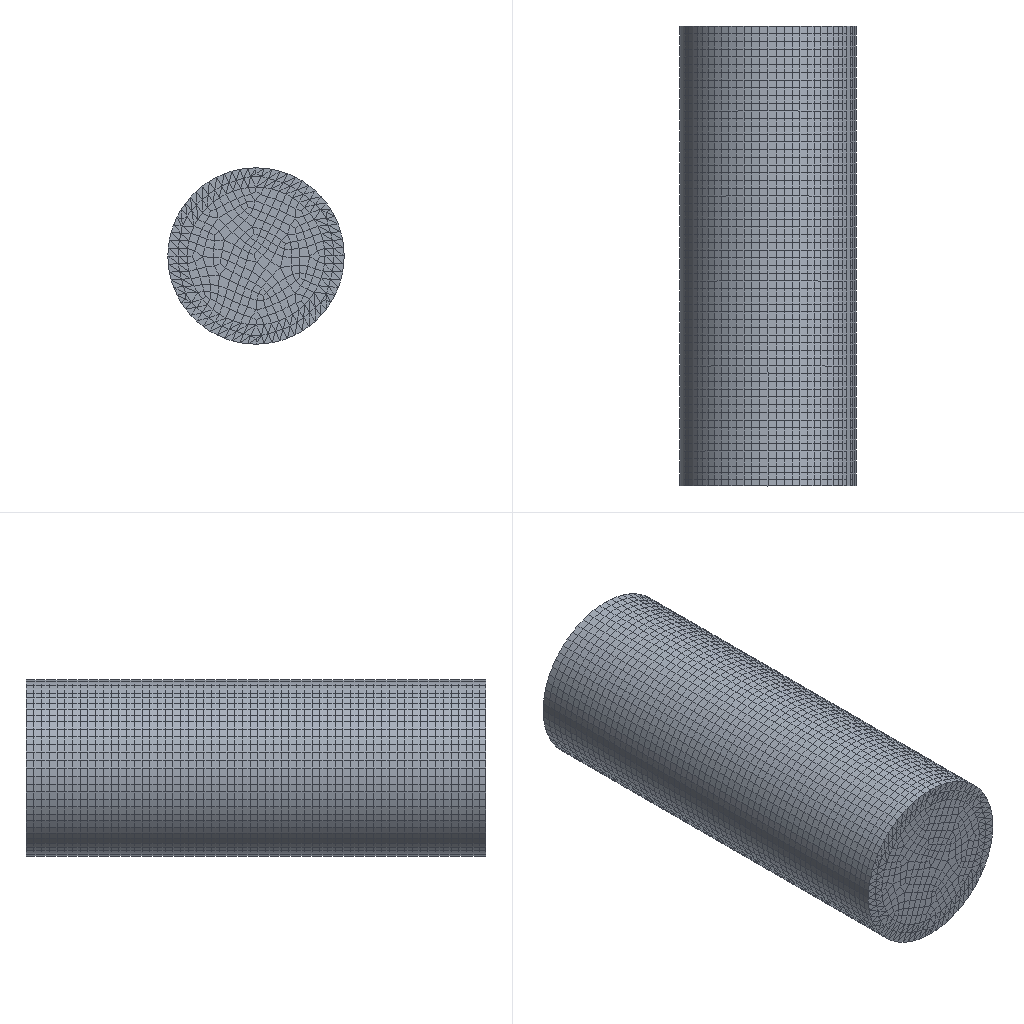Simulation study | ansys workbench
Ansys APDL input file, long lists of numbers shortened:
/batch
/config,noeldb,1     ! force off writing results to database
*get,_wallstrt,active,,time,wall
! ANSYS input file written by Workbench version 2020 R2
! File used for geometry attach:
/title,___ ___ _____--____ (B5)
*DIM,_wb_ProjectScratch_dir,string,248
_wb_ProjectScratch_dir(1) = ''
*DIM,_wb_SolverFiles_dir,string,248
_wb_SolverFiles_dir(1) = ''
*DIM,_wb_userfiles_dir,string,248
_wb_userfiles_dir(1) = ''
/com,--- Data in consistent NMM units. See Solving Units in the help system for more information.
/units,MPA
/nopr
/wb,file,start              !  signify a WB generated input file
/prep7
! Turn off shape checking because checks already performed inside WB mesher.
! See help system for more information.
SHPP,OFF,,NOWARN
/nolist
etcon,set             ! allow ANSYS to choose best KEYOP's for 180x elements
/com,*********** Nodes for the whole assembly ***********
nblock,3,,50740
(1i9,3e20.9e3)
        1    -1.192148224E+01     0.000000000E+00    -1.104059469E+01
! (46127 more lines like these left out)
-1
/com,*********** Nodes for all Remote Points ***********
nblock,3
(1i9,3e20.9e3)
    46129    -3.739912759E-16     0.000000000E+00    -5.749847455E-18
-1
/wb,elem,start            !  set before creation of elements
/com,*********** Elements for Body 1 "SYS\__" ***********
et,1,186
keyo,1,2,1          ! set full integration on SOLID186
eblock,19,solid,,8511
(19i9)
        1        1        1        1        0        0        0        0       20        0        1      424      532    12288    12285      422      531    12424    12421
! (17021 more lines like these left out)
-1
/wb,elem,end               !  done creating elements
/com,*********** Send User Defined Coordinate System(s) ***********
csys,0
toffst,273.15,  ! Temperature offset from absolute zero
/com,*********** Set Reference Temperature ***********
tref,22.
/wb,mat,start              !  starting to send materials
/com,*********** Send Materials ***********
Temperature = 'TEMP' ! Temperature
MP,DENS,1,7.85e-09,	! tonne mm^-3
MP,ALPX,1,1.2e-05,	! C^-1
MP,C,1,434000000,	! mm^2 s^-2 C^-1
MP,KXX,1,60.5,	! tonne mm s^-3 C^-1
MP,RSVX,1,0.00017,	! ohm mm
MP,EX,1,200000,	! tonne s^-2 mm^-1
MP,NUXY,1,0.3,
MP,MURX,1,10000,
/wb,mat,end                !  done sending materials
!************************* Model Summary ********************
!SYS\__,	Structural Steel,	matid,	1
!************************* End Model Summary ********************
! get the diagonal of the bounding box. Needed later for other things
*get,_xmin,node,,mnloc,x
*get,_ymin,node,,mnloc,y
*get,_zmin,node,,mnloc,z
*get,_xmax,node,,mxloc,x
*get,_ymax,node,,mxloc,y
*get,_zmax,node,,mxloc,z
_ASMDIAG=(_xmax-_xmin)*(_xmax-_xmin)+(_ymax-_ymin)*(_ymax-_ymin)+(_zmax-_zmin)*(_zmax-_zmin)
_ASMDIAG=SQRT(_ASMDIAG)
/wb,contact,start          !  starting to send contact
/wb,contact,end            !  done creating contacts
/golist
/wb,load,start             !  starting to send loads
/com,*********** Create Remote Point "内部远程点" ***********
! -------- Remote Point Used by "远程位移" --------
*set,tid,3
*set,cid,2
et,cid,174
et,tid,170
keyo,tid,2,1               ! Don't fix the pilot node
keyo,tid,4,111111
keyo,cid,12,5              ! Bonded Contact
keyo,cid,4,1               ! Deformable RBE3 style load
keyo,cid,2,2               ! MPC style contact
eblock,10,,,367
(15i9)
    16519        2        2        2        0      422      531    12424    12421    14069    46128    45807    46085
! (366 more lines like these left out)
-1
*set,_npilot,46129
_npilot95=_npilot
type,tid
mat ,cid
real,cid
tshape,pilo
en,16886,_npilot
tshape
/com,*********** Construct Remote Displacement ***********
/COM,*** Create a component for all remote displacements ***
CMBLOCK,REMOTEDISPALL,NODE,        1
(8i10)
     46129
/gst,on,on
fini
*get,_numnode,node,0,count
*get,_numelem,elem,0,count
*get, _MAXELEMNUM, elem, 0, NUM, MAX
*get, _MAXNODENUM, node, 0, NUM, MAX
*get, _MAXELEMTYPE, etyp, 0, NUM, MAX
*get, _MAXREALCONST, real, 0, NUM, MAX
/go
/wb,load,end               !  done creating loads
/com,--- Number of total nodes = %_numnode%
/com,--- Number of contact elements = 367
/com,--- Number of spring elements = 0
/com,--- Number of bearing elements = 0
/com,--- Number of solid elements = 8511
/com,--- Number of condensed parts = 0
/com,--- Number of total elements = %_numelem%
*get,_wallbsol,active,,time,wall
/com,****************************************************************************
/com,*************************    SOLUTION       ********************************
/com,****************************************************************************
/solu
antype,0                   ! static analysis
_thickRatio=  1     ! Ratio of thick parts in the model
eqsl,pcg,1e-8,,,,,,1
cntr,print,1               ! print out contact info and also make no initial contact an error
nldiag,cont,iter           ! print out contact info each equilibrium iteration
rescontrol,,none                 ! Do not keep any restart files
/com,****************************************************
/com,******************* SOLVE FOR LS 1 OF 1 ****************
d,46129,ux,0.
d,46129,uy,0.
d,46129,uz,0.
d,46129,rotx,0.
d,46129,roty,0.
d,46129,rotz,0.
acel,0.,9806.65,0.
/nopr
/gopr
/com,*********** Create Imported Load "________" ***********
/nopr
bf,1,temp,99.381
bf,2,temp,99.286
bf,3,temp,99.555
bf,4,temp,99.382
! (46124 more lines like these left out)
/gopr
nsub,1,1,1
time,1.
outres,erase
outres,all,none
outres,nsol,all,
outres,rsol,all
outres,eangl,all
outres,etmp,all
outres,veng,all
outres,strs,all,
outres,epel,all,
outres,eppl,all,
outres,epth,all,
outres,cont,all,
! *********** WB SOLVE COMMAND ***********
! check interactive state
*get,ANSINTER_,active,,int
*if,ANSINTER_,ne,0,then
/eof
*endif
solve
/com *************** Write FE CONNECTORS *********
CEWRITE,file,ce,,INTE
/com,****************************************************
/com,*************** FINISHED SOLVE FOR LS 1 *************
*get,_wallasol,active,,time,wall
/nopr
*get,_numnode,node,0,count
*get,_numelem,elem,0,count
*get, _MAXELEMNUM, elem, 0, NUM, MAX
*get, _MAXNODENUM, node, 0, NUM, MAX,,,INTERNAL
*get, _MAXELEMTYPE, etyp, 0, NUM, MAX
*get, _MAXREALCONST, real, 0, NUM, MAX
/gopr
*get,_PCGITER,active,,solu,cgiter
/post1
xmlo,ENCODING,ISO-8859-1
xmlo,parm
/xml,parm,xml
fini
/gopr
*get,_walldone,active,,time,wall
_preptime=(_wallbsol-_wallstrt)*3600
_solvtime=(_wallasol-_wallbsol)*3600
_posttime=(_walldone-_wallasol)*3600
_totaltim=(_walldone-_wallstrt)*3600
*get,_dlbratio,active,0,solu,dlbr
*get,_combtime,active,0,solu,comb
/com,--- Total number of nodes = %_numnode%
/com,--- Total number of elements = %_numelem%
/com,--- Element load balance ratio = %_dlbratio%
/com,--- Time to combine distributed files = %_combtime%
/wb,file,end               ! done with WB generated input